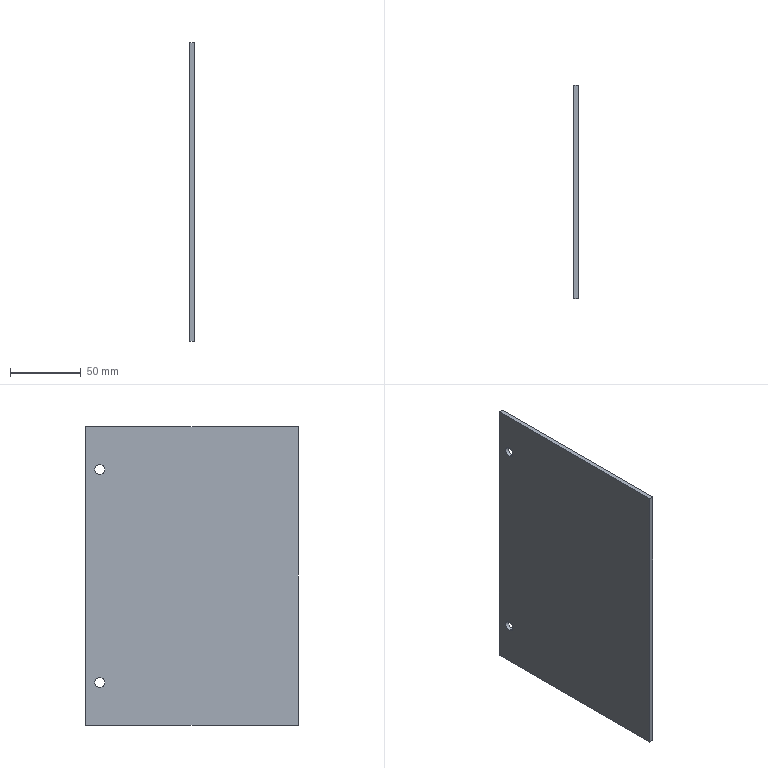Part | SolidWorks | features FlatPattern 1, HoleWzd 1, SMBaseFlange 1, SheetMetal 1 | 1 solid | 10 faces | box 3 x 150 x 210 mm | volume 94269 mm3 | plane 6 | cylinder 4 | commonest cylinder face diameters 7 x4
STEP:
#1=CARTESIAN_POINT('',(-3.,140.,-33.5));
#2=VERTEX_POINT('',#1);
#3=CARTESIAN_POINT('',(-3.,140.,-26.5));
#4=VERTEX_POINT('',#3);
#5=CARTESIAN_POINT('',(-3.,140.,-30.));
#6=DIRECTION('',(-1.,0.,0.));
#7=DIRECTION('',(0.,0.,1.));
#8=AXIS2_PLACEMENT_3D('',#5,#6,#7);
#9=CIRCLE('',#8,3.5);
#10=EDGE_CURVE('',#2,#4,#9,.T.);
#11=ORIENTED_EDGE('',*,*,#10,.T.);
#12=CARTESIAN_POINT('',(0.,140.,-26.5));
#13=VERTEX_POINT('',#12);
#14=CARTESIAN_POINT('',(0.,140.,-26.5));
#15=DIRECTION('',(1.,0.,0.));
#16=VECTOR('',#15,1000.);
#17=LINE('',#14,#16);
#18=EDGE_CURVE('',#4,#13,#17,.T.);
#19=ORIENTED_EDGE('',*,*,#18,.T.);
#20=CARTESIAN_POINT('',(0.,140.,-33.5));
#21=VERTEX_POINT('',#20);
#22=CARTESIAN_POINT('',(0.,140.,-30.));
#23=DIRECTION('',(1.,0.,0.));
#24=DIRECTION('',(0.,0.,-1.));
#25=AXIS2_PLACEMENT_3D('',#22,#23,#24);
#26=CIRCLE('',#25,3.5);
#27=EDGE_CURVE('',#13,#21,#26,.T.);
#28=ORIENTED_EDGE('',*,*,#27,.T.);
#29=CARTESIAN_POINT('',(0.,140.,-33.5));
#30=DIRECTION('',(1.,0.,0.));
#31=VECTOR('',#30,1000.);
#32=LINE('',#29,#31);
#33=EDGE_CURVE('',#2,#21,#32,.T.);
#34=ORIENTED_EDGE('',*,*,#33,.F.);
#35=EDGE_LOOP('',(#11,#19,#28,#34));
#36=FACE_OUTER_BOUND('',#35,.T.);
#37=CARTESIAN_POINT('',(0.,140.,-30.));
#38=DIRECTION('',(1.,0.,0.));
#39=DIRECTION('',(0.,0.,-1.));
#40=AXIS2_PLACEMENT_3D('',#37,#38,#39);
#41=CYLINDRICAL_SURFACE('',#40,3.5);
#42=ADVANCED_FACE('',(#36),#41,.F.);
#43=CARTESIAN_POINT('',(-3.,140.,-183.5));
#44=VERTEX_POINT('',#43);
#45=CARTESIAN_POINT('',(-3.,140.,-176.5));
#46=VERTEX_POINT('',#45);
#47=CARTESIAN_POINT('',(-3.,140.,-180.));
#48=DIRECTION('',(-1.,0.,0.));
#49=DIRECTION('',(0.,0.,1.));
#50=AXIS2_PLACEMENT_3D('',#47,#48,#49);
#51=CIRCLE('',#50,3.5);
#52=EDGE_CURVE('',#44,#46,#51,.T.);
#53=ORIENTED_EDGE('',*,*,#52,.T.);
#54=CARTESIAN_POINT('',(0.,140.,-176.5));
#55=VERTEX_POINT('',#54);
#56=CARTESIAN_POINT('',(0.,140.,-176.5));
#57=DIRECTION('',(1.,0.,0.));
#58=VECTOR('',#57,1000.);
#59=LINE('',#56,#58);
#60=EDGE_CURVE('',#46,#55,#59,.T.);
#61=ORIENTED_EDGE('',*,*,#60,.T.);
#62=CARTESIAN_POINT('',(0.,140.,-183.5));
#63=VERTEX_POINT('',#62);
#64=CARTESIAN_POINT('',(0.,140.,-180.));
#65=DIRECTION('',(1.,0.,0.));
#66=DIRECTION('',(0.,0.,-1.));
#67=AXIS2_PLACEMENT_3D('',#64,#65,#66);
#68=CIRCLE('',#67,3.5);
#69=EDGE_CURVE('',#55,#63,#68,.T.);
#70=ORIENTED_EDGE('',*,*,#69,.T.);
#71=CARTESIAN_POINT('',(0.,140.,-183.5));
#72=DIRECTION('',(1.,0.,0.));
#73=VECTOR('',#72,1000.);
#74=LINE('',#71,#73);
#75=EDGE_CURVE('',#44,#63,#74,.T.);
#76=ORIENTED_EDGE('',*,*,#75,.F.);
#77=EDGE_LOOP('',(#53,#61,#70,#76));
#78=FACE_OUTER_BOUND('',#77,.T.);
#79=CARTESIAN_POINT('',(0.,140.,-180.));
#80=DIRECTION('',(1.,0.,0.));
#81=DIRECTION('',(0.,0.,-1.));
#82=AXIS2_PLACEMENT_3D('',#79,#80,#81);
#83=CYLINDRICAL_SURFACE('',#82,3.5);
#84=ADVANCED_FACE('',(#78),#83,.F.);
#85=CARTESIAN_POINT('',(0.,150.,0.));
#86=VERTEX_POINT('',#85);
#87=CARTESIAN_POINT('',(0.,0.,0.));
#88=VERTEX_POINT('',#87);
#89=CARTESIAN_POINT('',(0.,0.,0.));
#90=DIRECTION('',(0.,-1.,0.));
#91=VECTOR('',#90,1000.);
#92=LINE('',#89,#91);
#93=EDGE_CURVE('',#86,#88,#92,.T.);
#94=ORIENTED_EDGE('',*,*,#93,.F.);
#95=CARTESIAN_POINT('',(-3.,150.,0.));
#96=VERTEX_POINT('',#95);
#97=CARTESIAN_POINT('',(-3.,150.,0.));
#98=DIRECTION('',(1.,0.,0.));
#99=VECTOR('',#98,1000.);
#100=LINE('',#97,#99);
#101=EDGE_CURVE('',#96,#86,#100,.T.);
#102=ORIENTED_EDGE('',*,*,#101,.F.);
#103=CARTESIAN_POINT('',(-3.,0.,0.));
#104=VERTEX_POINT('',#103);
#105=CARTESIAN_POINT('',(-3.,0.,0.));
#106=DIRECTION('',(0.,-1.,0.));
#107=VECTOR('',#106,1000.);
#108=LINE('',#105,#107);
#109=EDGE_CURVE('',#96,#104,#108,.T.);
#110=ORIENTED_EDGE('',*,*,#109,.T.);
#111=CARTESIAN_POINT('',(-3.,0.,0.));
#112=DIRECTION('',(1.,0.,0.));
#113=VECTOR('',#112,1000.);
#114=LINE('',#111,#113);
#115=EDGE_CURVE('',#104,#88,#114,.T.);
#116=ORIENTED_EDGE('',*,*,#115,.T.);
#117=EDGE_LOOP('',(#94,#102,#110,#116));
#118=FACE_OUTER_BOUND('',#117,.T.);
#119=CARTESIAN_POINT('',(-3.,0.,0.));
#120=DIRECTION('',(0.,0.,1.));
#121=DIRECTION('',(1.,0.,0.));
#122=AXIS2_PLACEMENT_3D('',#119,#120,#121);
#123=PLANE('',#122);
#124=ADVANCED_FACE('',(#118),#123,.T.);
#125=CARTESIAN_POINT('',(0.,150.,-210.));
#126=VERTEX_POINT('',#125);
#127=CARTESIAN_POINT('',(0.,150.,0.));
#128=DIRECTION('',(0.,0.,1.));
#129=VECTOR('',#128,1000.);
#130=LINE('',#127,#129);
#131=EDGE_CURVE('',#126,#86,#130,.T.);
#132=ORIENTED_EDGE('',*,*,#131,.F.);
#133=CARTESIAN_POINT('',(-3.,150.,-210.));
#134=VERTEX_POINT('',#133);
#135=CARTESIAN_POINT('',(-3.,150.,-210.));
#136=DIRECTION('',(1.,0.,0.));
#137=VECTOR('',#136,1000.);
#138=LINE('',#135,#137);
#139=EDGE_CURVE('',#134,#126,#138,.T.);
#140=ORIENTED_EDGE('',*,*,#139,.F.);
#141=CARTESIAN_POINT('',(-3.,150.,0.));
#142=DIRECTION('',(0.,0.,1.));
#143=VECTOR('',#142,1000.);
#144=LINE('',#141,#143);
#145=EDGE_CURVE('',#134,#96,#144,.T.);
#146=ORIENTED_EDGE('',*,*,#145,.T.);
#147=ORIENTED_EDGE('',*,*,#101,.T.);
#148=EDGE_LOOP('',(#132,#140,#146,#147));
#149=FACE_OUTER_BOUND('',#148,.T.);
#150=CARTESIAN_POINT('',(-3.,150.,0.));
#151=DIRECTION('',(0.,1.,0.));
#152=DIRECTION('',(0.,0.,1.));
#153=AXIS2_PLACEMENT_3D('',#150,#151,#152);
#154=PLANE('',#153);
#155=ADVANCED_FACE('',(#149),#154,.T.);
#156=CARTESIAN_POINT('',(0.,0.,-210.));
#157=VERTEX_POINT('',#156);
#158=CARTESIAN_POINT('',(0.,150.,-210.));
#159=DIRECTION('',(0.,1.,0.));
#160=VECTOR('',#159,1000.);
#161=LINE('',#158,#160);
#162=EDGE_CURVE('',#157,#126,#161,.T.);
#163=ORIENTED_EDGE('',*,*,#162,.F.);
#164=CARTESIAN_POINT('',(-3.,0.,-210.));
#165=VERTEX_POINT('',#164);
#166=CARTESIAN_POINT('',(-3.,0.,-210.));
#167=DIRECTION('',(1.,0.,0.));
#168=VECTOR('',#167,1000.);
#169=LINE('',#166,#168);
#170=EDGE_CURVE('',#165,#157,#169,.T.);
#171=ORIENTED_EDGE('',*,*,#170,.F.);
#172=CARTESIAN_POINT('',(-3.,150.,-210.));
#173=DIRECTION('',(0.,1.,0.));
#174=VECTOR('',#173,1000.);
#175=LINE('',#172,#174);
#176=EDGE_CURVE('',#165,#134,#175,.T.);
#177=ORIENTED_EDGE('',*,*,#176,.T.);
#178=ORIENTED_EDGE('',*,*,#139,.T.);
#179=EDGE_LOOP('',(#163,#171,#177,#178));
#180=FACE_OUTER_BOUND('',#179,.T.);
#181=CARTESIAN_POINT('',(-3.,150.,-210.));
#182=DIRECTION('',(0.,0.,-1.));
#183=DIRECTION('',(0.,1.,0.));
#184=AXIS2_PLACEMENT_3D('',#181,#182,#183);
#185=PLANE('',#184);
#186=ADVANCED_FACE('',(#180),#185,.T.);
#187=CARTESIAN_POINT('',(0.,0.,0.));
#188=DIRECTION('',(0.,0.,-1.));
#189=VECTOR('',#188,1000.);
#190=LINE('',#187,#189);
#191=EDGE_CURVE('',#88,#157,#190,.T.);
#192=ORIENTED_EDGE('',*,*,#191,.F.);
#193=ORIENTED_EDGE('',*,*,#115,.F.);
#194=CARTESIAN_POINT('',(-3.,0.,0.));
#195=DIRECTION('',(0.,0.,-1.));
#196=VECTOR('',#195,1000.);
#197=LINE('',#194,#196);
#198=EDGE_CURVE('',#104,#165,#197,.T.);
#199=ORIENTED_EDGE('',*,*,#198,.T.);
#200=ORIENTED_EDGE('',*,*,#170,.T.);
#201=EDGE_LOOP('',(#192,#193,#199,#200));
#202=FACE_OUTER_BOUND('',#201,.T.);
#203=CARTESIAN_POINT('',(-3.,0.,0.));
#204=DIRECTION('',(0.,-1.,0.));
#205=DIRECTION('',(0.,0.,-1.));
#206=AXIS2_PLACEMENT_3D('',#203,#204,#205);
#207=PLANE('',#206);
#208=ADVANCED_FACE('',(#202),#207,.T.);
#209=ORIENTED_EDGE('',*,*,#10,.F.);
#210=CARTESIAN_POINT('',(-3.,140.,-30.));
#211=DIRECTION('',(-1.,0.,0.));
#212=DIRECTION('',(0.,0.,1.));
#213=AXIS2_PLACEMENT_3D('',#210,#211,#212);
#214=CIRCLE('',#213,3.5);
#215=EDGE_CURVE('',#4,#2,#214,.T.);
#216=ORIENTED_EDGE('',*,*,#215,.F.);
#217=EDGE_LOOP('',(#209,#216));
#218=FACE_BOUND('',#217,.T.);
#219=ORIENTED_EDGE('',*,*,#52,.F.);
#220=CARTESIAN_POINT('',(-3.,140.,-180.));
#221=DIRECTION('',(-1.,0.,0.));
#222=DIRECTION('',(0.,0.,1.));
#223=AXIS2_PLACEMENT_3D('',#220,#221,#222);
#224=CIRCLE('',#223,3.5);
#225=EDGE_CURVE('',#46,#44,#224,.T.);
#226=ORIENTED_EDGE('',*,*,#225,.F.);
#227=EDGE_LOOP('',(#219,#226));
#228=FACE_BOUND('',#227,.T.);
#229=ORIENTED_EDGE('',*,*,#109,.F.);
#230=ORIENTED_EDGE('',*,*,#145,.F.);
#231=ORIENTED_EDGE('',*,*,#176,.F.);
#232=ORIENTED_EDGE('',*,*,#198,.F.);
#233=EDGE_LOOP('',(#229,#230,#231,#232));
#234=FACE_OUTER_BOUND('',#233,.T.);
#235=CARTESIAN_POINT('',(-3.,0.,0.));
#236=DIRECTION('',(-1.,0.,0.));
#237=DIRECTION('',(0.,0.,1.));
#238=AXIS2_PLACEMENT_3D('',#235,#236,#237);
#239=PLANE('',#238);
#240=ADVANCED_FACE('',(#218,#228,#234),#239,.T.);
#241=CARTESIAN_POINT('',(0.,140.,-30.));
#242=DIRECTION('',(1.,0.,0.));
#243=DIRECTION('',(0.,0.,-1.));
#244=AXIS2_PLACEMENT_3D('',#241,#242,#243);
#245=CIRCLE('',#244,3.5);
#246=EDGE_CURVE('',#21,#13,#245,.T.);
#247=ORIENTED_EDGE('',*,*,#246,.F.);
#248=ORIENTED_EDGE('',*,*,#27,.F.);
#249=EDGE_LOOP('',(#247,#248));
#250=FACE_BOUND('',#249,.T.);
#251=CARTESIAN_POINT('',(0.,140.,-180.));
#252=DIRECTION('',(1.,0.,0.));
#253=DIRECTION('',(0.,0.,-1.));
#254=AXIS2_PLACEMENT_3D('',#251,#252,#253);
#255=CIRCLE('',#254,3.5);
#256=EDGE_CURVE('',#63,#55,#255,.T.);
#257=ORIENTED_EDGE('',*,*,#256,.F.);
#258=ORIENTED_EDGE('',*,*,#69,.F.);
#259=EDGE_LOOP('',(#257,#258));
#260=FACE_BOUND('',#259,.T.);
#261=ORIENTED_EDGE('',*,*,#93,.T.);
#262=ORIENTED_EDGE('',*,*,#191,.T.);
#263=ORIENTED_EDGE('',*,*,#162,.T.);
#264=ORIENTED_EDGE('',*,*,#131,.T.);
#265=EDGE_LOOP('',(#261,#262,#263,#264));
#266=FACE_OUTER_BOUND('',#265,.T.);
#267=CARTESIAN_POINT('',(0.,0.,0.));
#268=DIRECTION('',(-1.,0.,0.));
#269=DIRECTION('',(0.,0.,1.));
#270=AXIS2_PLACEMENT_3D('',#267,#268,#269);
#271=PLANE('',#270);
#272=ADVANCED_FACE('',(#250,#260,#266),#271,.F.);
#273=ORIENTED_EDGE('',*,*,#60,.F.);
#274=ORIENTED_EDGE('',*,*,#225,.T.);
#275=ORIENTED_EDGE('',*,*,#75,.T.);
#276=ORIENTED_EDGE('',*,*,#256,.T.);
#277=EDGE_LOOP('',(#273,#274,#275,#276));
#278=FACE_OUTER_BOUND('',#277,.T.);
#279=CARTESIAN_POINT('',(0.,140.,-180.));
#280=DIRECTION('',(1.,0.,0.));
#281=DIRECTION('',(0.,0.,-1.));
#282=AXIS2_PLACEMENT_3D('',#279,#280,#281);
#283=CYLINDRICAL_SURFACE('',#282,3.5);
#284=ADVANCED_FACE('',(#278),#283,.F.);
#285=ORIENTED_EDGE('',*,*,#18,.F.);
#286=ORIENTED_EDGE('',*,*,#215,.T.);
#287=ORIENTED_EDGE('',*,*,#33,.T.);
#288=ORIENTED_EDGE('',*,*,#246,.T.);
#289=EDGE_LOOP('',(#285,#286,#287,#288));
#290=FACE_OUTER_BOUND('',#289,.T.);
#291=CARTESIAN_POINT('',(0.,140.,-30.));
#292=DIRECTION('',(1.,0.,0.));
#293=DIRECTION('',(0.,0.,-1.));
#294=AXIS2_PLACEMENT_3D('',#291,#292,#293);
#295=CYLINDRICAL_SURFACE('',#294,3.5);
#296=ADVANCED_FACE('',(#290),#295,.F.);
#297=CLOSED_SHELL('',(#42,#84,#124,#155,#186,#208,#240,#272,#284,#296));
#298=MANIFOLD_SOLID_BREP('',#297);
#299=CARTESIAN_POINT('',(0.,0.,0.));
#300=DIRECTION('',(0.,0.,1.));
#301=DIRECTION('',(1.,0.,0.));
#302=AXIS2_PLACEMENT_3D('',#299,#300,#301);
#303=(LENGTH_UNIT()NAMED_UNIT(*)SI_UNIT(.MILLI.,.METRE.));
#304=UNCERTAINTY_MEASURE_WITH_UNIT(LENGTH_MEASURE(0.00001),#303,'','');
#305=(NAMED_UNIT(*)PLANE_ANGLE_UNIT()SI_UNIT($,.RADIAN.));
#306=(NAMED_UNIT(*)SI_UNIT($,.STERADIAN.)SOLID_ANGLE_UNIT());
#307=(GEOMETRIC_REPRESENTATION_CONTEXT(3)GLOBAL_UNCERTAINTY_ASSIGNED_CONTEXT((#304))GLOBAL_UNIT_ASSIGNED_CONTEXT((#303,#305,#306))REPRESENTATION_CONTEXT('',''));
#308=ADVANCED_BREP_SHAPE_REPRESENTATION('',(#298,#302),#307);